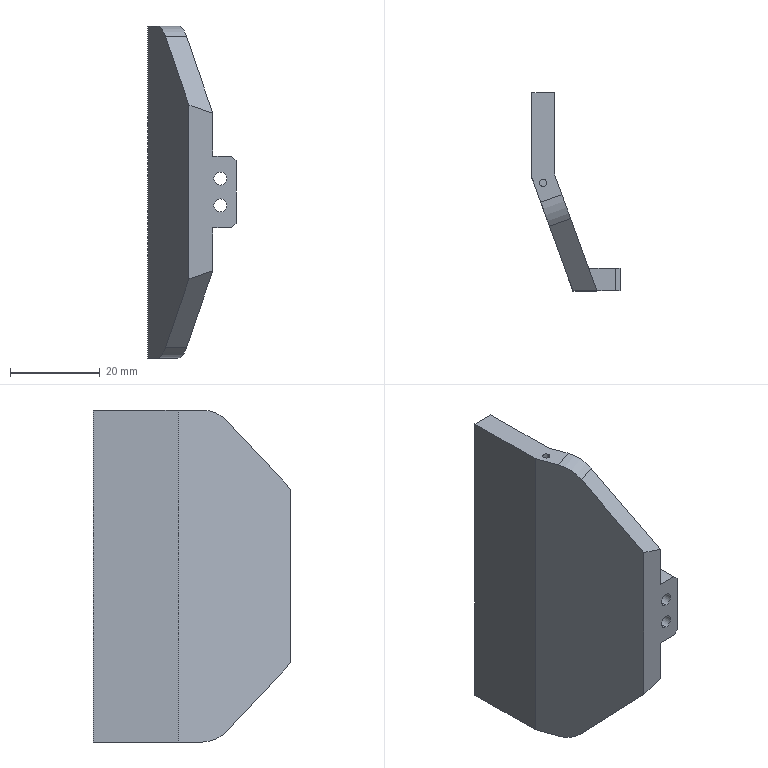NC program | NX | posted with a generic post | part box 19.643 x 44.061 x 74 mm
Lines 614 to 1768 of 4832:
(CURVE_DRIVE , TOOL : R1)
N1202 T04 M6
N1204 G54
N1206 G17 G0 G90 X15.026 Y-7.76 B0. C0. S6500 M3
N1208 G43 Z29.368 H4
N1210 Z2.364
N1212 G94 G1 Z0.531 F2500.
N1214 Y-7.722 Z0.393
N1216 Y-7.705 Z0.252
N1218 Y-7.708 Z0.109
N1220 Y-7.731 Z-0.032
N1222 Y-7.774 Z-0.168
N1224 Y-7.836 Z-0.296
N1226 Y-7.915 Z-0.415
N1228 Y-8.011 Z-0.521
N1230 Y-8.121 Z-0.612
N1232 Y-8.242 Z-0.687
N1234 Y-8.373 Z-0.743
N1236 Y-8.42 Z-0.76
N1238 X15.006 Z-0.768
N1240 X14.979 Y-8.401 Z-0.771
N1242 Y-8.348 Z-0.751
N1244 Y-8.326 Z-0.743
N1246 X14.932 Y-8.279
N1248 Y-8.302 Z-0.751
N1250 Y-8.367 Z-0.776
N1252 X14.885 Y-8.334 Z-0.782
N1254 Y-8.256 Z-0.752
N1256 Y-8.232 Z-0.743
N1258 X14.837 Y-8.185
N1260 Y-8.236 Z-0.762
N1262 Y-8.302 Z-0.787
N1264 X14.79 Y-8.27 Z-0.792
N1266 Y-8.162 Z-0.752
N1268 Y-8.137 Z-0.743
N1270 X14.743 Y-8.09
N1272 Y-8.239 Z-0.797
N1274 X14.696 Y-8.207 Z-0.803
N1276 Y-8.043 Z-0.743
N1278 X14.648 Y-7.995
N1280 Y-8.178 Z-0.81
N1282 X14.601 Y-8.149 Z-0.817
N1284 Y-7.948 Z-0.743
N1286 X14.554 Y-7.901
N1288 Y-8.12 Z-0.823
N1290 X14.507 Y-8.092 Z-0.831
N1292 Y-8.036 Z-0.809
N1294 Y-7.854 Z-0.743
N1296 X14.459 Y-7.806
N1298 Y-7.989 Z-0.81
N1300 Y-8.065 Z-0.838
N1302 X14.412 Y-8.038 Z-0.845
N1304 Y-7.943 Z-0.81
N1306 Y-7.759 Z-0.743
N1308 X14.365 Y-7.712
N1310 Y-7.931 Z-0.823
N1312 Y-8.013 Z-0.853
N1314 X14.318 Y-7.989 Z-0.862
N1316 Y-7.931 Z-0.84
N1318 Y-7.665 Z-0.743
N1320 X14.27 Y-7.617
N1322 Y-7.956 Z-0.866
N1324 Y-7.964 Z-0.87
N1326 X14.223 Y-7.94 Z-0.878
N1328 Y-7.909 Z-0.866
N1330 Y-7.57 Z-0.743
N1332 X14.176 Y-7.523
N1334 Y-7.863 Z-0.867
N1336 Y-7.917 Z-0.887
N1338 X14.129 Y-7.894 Z-0.896
N1340 Y-7.816 Z-0.867
N1342 Y-7.476 Z-0.743
N1344 X14.082 Y-7.428
N1346 Y-7.779 Z-0.87
N1348 Y-7.872 Z-0.906
N1350 X14.034 Y-7.851 Z-0.915
N1352 Y-7.779 Z-0.888
N1354 Y-7.381 Z-0.743
N1356 X13.987 Y-7.334
N1358 Y-7.779 Z-0.905
N1360 Y-7.831 Z-0.925
N1362 X13.94 Y-7.81 Z-0.934
N1364 Y-7.779 Z-0.922
N1366 Y-7.287 Z-0.743
N1368 X13.892 Y-7.239
N1370 Y-7.791 Z-0.944
N1372 X13.845 Y-7.771 Z-0.954
N1374 Y-7.192 Z-0.743
N1376 X13.798 Y-7.145
N1378 Y-7.643 Z-0.924
N1380 Y-7.752 Z-0.965
N1382 X13.779 Y-7.744 Z-0.969
N1384 X13.751 Y-7.734 Z-0.975
N1386 Y-7.097 Z-0.743
N1388 X13.703 Y-7.05
N1390 Y-7.718 Z-0.986
N1392 X13.656 Y-7.701 Z-0.997
N1394 Y-7.003 Z-0.743
N1396 X13.609 Y-6.956
N1398 Y-7.685 Z-1.008
N1400 X13.561 Y-7.669 Z-1.02
N1402 Y-6.908 Z-0.743
N1404 X13.514 Y-6.861
N1406 Y-7.654 Z-1.032
N1408 X13.467 Y-7.639 Z-1.044
N1410 Y-7.626 Z-1.039
N1412 Y-6.814 Z-0.743
N1414 X13.42 Y-6.766
N1416 Y-7.625 Z-1.056
N1418 X13.372 Y-7.61 Z-1.068
N1420 Y-6.719 Z-0.743
N1422 X13.325 Y-6.672
N1424 Y-7.486 Z-1.039
N1426 Y-7.596 Z-1.08
N1428 X13.303 Y-7.59 Z-1.086
N1430 X13.278 Y-7.584 Z-1.092
N1432 Y-6.625 Z-0.743
N1434 X13.231 Y-6.577
N1436 Y-7.572 Z-1.105
N1438 X13.183 Y-7.561 Z-1.118
N1440 Y-6.53 Z-0.743
N1442 X13.136 Y-6.483
N1444 Y-7.549 Z-1.131
N1446 X13.089 Y-7.539 Z-1.145
N1448 Y-6.435 Z-0.743
N1450 X13.041 Y-6.388
N1452 Y-7.474 Z-1.138
N1454 Y-7.528 Z-1.158
N1456 X12.994 Y-7.518 Z-1.172
N1458 Y-6.341 Z-0.743
N1460 X12.947 Y-6.294
N1462 Y-7.509 Z-1.186
N1464 X12.899 Y-7.5 Z-1.2
N1466 Y-6.246 Z-0.743
N1468 X12.852 Y-6.199
N1470 Y-7.474 Z-1.207
N1472 Y-7.492 Z-1.214
N1474 X12.805 Y-7.484 Z-1.228
N1476 Y-6.152 Z-0.743
N1478 X12.758 Y-6.104
N1480 Y-7.477 Z-1.243
N1482 X12.71 Y-7.469 Z-1.257
N1484 Y-6.102 Z-0.759
N1486 Y-6.057 Z-0.744
N1488 X12.663 Y-6.01 Z-0.743
N1490 Y-6.102 Z-0.776
N1492 Y-7.463 Z-1.272
N1494 X12.616 Y-7.457 Z-1.287
N1496 Y-5.963 Z-0.743
N1498 X12.568 Y-5.915 Z-0.744
N1500 Y-5.949 Z-0.755
N1502 Y-7.451 Z-1.302
N1504 X12.521 Y-7.445 Z-1.317
N1506 Y-5.928 Z-0.765
N1508 Y-5.867 Z-0.744
N1510 X12.474 Y-5.82
N1512 Y-5.882 Z-0.765
N1514 Y-7.406 Z-1.32
N1516 Y-7.441 Z-1.333
N1518 X12.427 Y-7.436 Z-1.349
N1520 Y-7.321 Z-1.306
N1522 Y-5.835 Z-0.766
N1524 Y-5.773 Z-0.744
N1526 X12.379 Y-5.726
N1528 Y-5.789 Z-0.766
N1530 Y-7.321 Z-1.324
N1532 Y-7.432 Z-1.365
N1534 X12.332 Y-7.429 Z-1.381
N1536 Y-7.321 Z-1.341
N1538 Y-5.742 Z-0.766
N1540 Y-5.678 Z-0.744
N1542 X12.285 Y-5.631
N1544 Y-5.696 Z-0.766
N1546 Y-7.373 Z-1.377
N1548 Y-7.426 Z-1.397
N1550 X12.238 Y-7.424 Z-1.413
N1552 Y-7.325 Z-1.377
N1554 Y-5.65 Z-0.767
N1556 Y-5.584 Z-0.744
N1558 X12.191 Y-5.537
N1560 Y-5.603 Z-0.767
N1562 Y-7.321 Z-1.392
N1564 Y-7.422 Z-1.43
N1566 X12.144 Y-7.42 Z-1.447
N1568 Y-7.321 Z-1.409
N1570 Y-5.557 Z-0.767
N1572 Y-5.49 Z-0.744
N1574 X12.096 Y-5.443
N1576 Y-5.51 Z-0.767
N1578 Y-7.34 Z-1.433
N1580 Y-7.419 Z-1.463
N1582 X12.049 Y-7.418 Z-1.48
N1584 Y-7.321 Z-1.444
N1586 Y-5.464 Z-0.768
N1588 Y-5.395 Z-0.744
N1590 X12.002 Y-5.348
N1592 Y-5.417 Z-0.768
N1594 Y-7.321 Z-1.461
N1596 Y-7.417 Z-1.497
N1598 X11.955 Z-1.514
N1600 Y-7.321 Z-1.478
N1602 Y-5.371 Z-0.768
N1604 Y-5.301 Z-0.744
N1606 X11.907 Y-5.254
N1608 Y-5.324 Z-0.768
N1610 Y-7.321 Z-1.495
N1612 Y-7.416 Z-1.531
N1614 X11.86 Z-1.548
N1616 Y-7.321 Z-1.513
N1618 Y-5.278 Z-0.769
N1620 Y-5.206 Z-0.744
N1622 X11.813 Y-5.159
N1624 Y-5.231 Z-0.769
N1626 Y-7.321 Z-1.53
N1628 Y-7.416 Z-1.566
N1630 X11.766 Z-1.583
N1632 Y-7.321 Z-1.547
N1634 Y-5.184 Z-0.769
N1636 Y-5.112 Z-0.744
N1638 X11.718 Y-5.064
N1640 Y-5.138 Z-0.769
N1642 Y-7.321 Z-1.564
N1644 Y-7.416 Z-1.6
N1646 X11.671 Z-1.617
N1648 Y-7.321 Z-1.581
N1650 Y-5.091 Z-0.77
N1652 Y-5.017 Z-0.744
N1654 X11.624 Y-4.97
N1656 Y-5.045 Z-0.77
N1658 Y-7.321 Z-1.599
N1660 Y-7.416 Z-1.634
N1662 X11.576 Z-1.652
N1664 Y-7.321 Z-1.616
N1666 Y-4.998 Z-0.77
N1668 Y-4.922 Z-0.744
N1670 X11.529 Y-4.875
N1672 Y-4.952 Z-0.771
N1674 Y-7.321 Z-1.633
N1676 Y-7.416 Z-1.669
N1678 X11.482 Z-1.686
N1680 Y-7.321 Z-1.65
N1682 Y-4.905 Z-0.771
N1684 Y-4.828 Z-0.744
N1686 X11.435 Y-4.781
N1688 Y-4.859 Z-0.771
N1690 Y-7.321 Z-1.667
N1692 Y-7.416 Z-1.703
N1694 X11.387 Y-7.417 Z-1.72
N1696 Y-7.321 Z-1.684
N1698 Y-4.812 Z-0.771
N1700 Y-4.734 Z-0.744
N1702 X11.353 Y-4.699 Z-0.743
N1704 X11.341 Y-4.685
N1706 Y-4.766 Z-0.771
N1708 Y-6.434 Z-1.378
N1710 Y-7.321 Z-1.701
N1712 Y-7.417 Z-1.737
N1714 X11.293 Y-7.418 Z-1.753
N1716 Y-7.321 Z-1.717
N1718 Y-5.106 Z-0.911
N1720 Y-4.719 Z-0.771
N1722 Y-4.63 Z-0.739
N1724 X11.246 Y-4.577 Z-0.735
N1726 Y-4.825 Z-0.825
N1728 Y-7.321 Z-1.733
N1730 Y-7.419 Z-1.769
N1732 X11.198 Y-7.42 Z-1.785
N1734 Y-7.321 Z-1.748
N1736 Y-4.626 Z-0.768
N1738 Y-4.526 Z-0.732
N1740 X11.151 Y-4.476 Z-0.729
N1742 Y-4.579 Z-0.766
N1744 Y-7.323 Z-1.765
N1746 Y-7.42 Z-1.801
N1748 X11.103 Y-7.422 Z-1.815
N1750 Y-7.321 Z-1.777
N1752 Y-6.559 Z-1.5
N1754 Y-6.407 Z-1.445
N1756 Y-6.361 Z-1.428
N1758 Y-4.532 Z-0.762
N1760 Y-4.429 Z-0.725
N1762 X11.078 Y-4.404
N1764 X11.063 Y-4.391
N1766 X11.055 Y-4.383 Z-0.724
N1768 Y-4.395 Z-0.728
N1770 Y-4.425 Z-0.737
N1772 Y-6.314 Z-1.424
N1774 Y-6.374 Z-1.447
N1776 Y-6.559 Z-1.513
N1778 Y-7.321 Z-1.791
N1780 Y-7.423 Z-1.829
N1782 X11.006 Y-7.424 Z-1.842
N1784 Y-7.321 Z-1.804
N1786 Y-4.425 Z-0.75
N1788 Y-4.34 Z-0.721
N1790 X10.982 Y-4.319 Z-0.719
N1792 X10.958 Y-4.3 Z-0.717
N1794 Y-4.389 Z-0.749
N1796 Y-7.321 Z-1.816
N1798 Y-7.425 Z-1.855
N1800 X10.909 Y-7.426 Z-1.866
N1802 Y-7.321 Z-1.827
N1804 Y-4.342 Z-0.743
N1806 Y-4.261 Z-0.715
N1808 X10.861 Y-4.223 Z-0.712
N1810 Y-7.321 Z-1.839
N1812 Y-7.427 Z-1.878
N1814 X10.828 Z-1.886
N1816 X10.812 Y-7.428 Z-1.889
N1818 Y-7.321 Z-1.849
N1820 Y-4.189 Z-0.71
N1822 X10.763 Y-4.158 Z-0.708
N1824 Y-7.321 Z-1.859
N1826 Y-7.428 Z-1.898
N1828 X10.714 Y-7.429 Z-1.908
N1830 Y-7.321 Z-1.868
N1832 Y-4.127 Z-0.706
N1834 X10.671 Y-4.1 Z-0.704
N1836 X10.665 Y-4.097
N1838 Y-4.12 Z-0.711
N1840 Y-7.321 Z-1.877
N1842 Y-7.43 Z-1.917
N1844 X10.615 Z-1.925
N1846 Y-7.321 Z-1.884
N1848 Y-4.12 Z-0.719
N1850 Y-4.072 Z-0.703
N1852 X10.595 Y-4.062 Z-0.702
N1854 X10.566 Y-4.049 Z-0.701
N1856 Y-4.12 Z-0.726
N1858 Y-7.321 Z-1.891
N1860 Y-7.431 Z-1.932
N1862 X10.518 Y-7.432 Z-1.939
N1864 X10.516
N1866 Y-7.321 Z-1.898
N1868 Y-4.12 Z-0.733
N1870 Y-4.028 Z-0.7
N1872 X10.467 Y-4.011
N1874 Y-4.12 Z-0.738
N1876 Y-7.321 Z-1.903
N1878 Y-7.432 Z-1.944
N1880 X10.417 Z-1.949
N1882 Y-7.321 Z-1.908
N1884 Y-4.12 Z-0.743
N1886 Y-3.994 Z-0.698
N1888 X10.367 Y-3.977 Z-0.696
N1890 Y-7.321 Z-1.913
N1892 Y-7.433 Z-1.954
N1894 X10.317 Z-1.958
N1896 Y-7.321 Z-1.916
N1898 Y-3.965 Z-0.695
N1900 X10.267 Y-3.952 Z-0.694
N1902 Y-7.321 Z-1.919
N1904 Y-7.433 Z-1.961
N1906 X10.218 Y-7.434 Z-1.964
N1908 Y-7.321 Z-1.922
N1910 Y-3.967 Z-0.702
N1912 Y-3.944 Z-0.694
N1914 X10.209 Y-3.943
N1916 X10.168 Y-3.941
N1918 Y-7.321 Z-1.924
N1920 Y-7.434 Z-1.965
N1922 X10.118 Z-1.967
N1924 Y-7.321 Z-1.925
N1926 Y-3.938 Z-0.694
N1928 X10.068 Y-3.936 Z-0.695
N1930 Y-3.967 Z-0.706
N1932 Y-7.324 Z-1.927
N1934 Y-7.434 Z-1.968
N1936 X10.018
N1938 Y-7.321 Z-1.927
N1940 Y-3.967 Z-0.706
N1942 Y-3.935 Z-0.695
N1944 X9.968
N1946 Y-3.967 Z-0.706
N1948 Y-7.321 Z-1.927
N1950 Y-7.434 Z-1.968
N1952 X9.918
N1954 Y-7.321 Z-1.927
N1956 Y-3.967 Z-0.706
N1958 Y-3.935 Z-0.695
N1960 X9.868
N1962 Y-3.967 Z-0.706
N1964 Y-7.321 Z-1.927
N1966 Y-7.434 Z-1.968
N1968 X9.818
N1970 Y-7.321 Z-1.927
N1972 Y-3.967 Z-0.706
N1974 Y-3.935 Z-0.695
N1976 X9.768
N1978 Y-3.967 Z-0.706
N1980 Y-7.321 Z-1.927
N1982 Y-7.434 Z-1.968
N1984 X9.718
N1986 Y-7.321 Z-1.927
N1988 Y-3.967 Z-0.706
N1990 Y-3.935 Z-0.695
N1992 X9.668
N1994 Y-3.967 Z-0.706
N1996 Y-7.321 Z-1.927
N1998 Y-7.434 Z-1.968
N2000 X9.618
N2002 Y-7.321 Z-1.927
N2004 Y-3.967 Z-0.706
N2006 Y-3.935 Z-0.695
N2008 X9.568
N2010 Y-3.967 Z-0.706
N2012 Y-7.321 Z-1.927
N2014 Y-7.434 Z-1.968
N2016 X9.518
N2018 Y-7.321 Z-1.927
N2020 Y-3.967 Z-0.706
N2022 Y-3.935 Z-0.695
N2024 X9.468
N2026 Y-3.967 Z-0.706
N2028 Y-7.321 Z-1.927
N2030 Y-7.434 Z-1.968
N2032 X9.418
N2034 Y-7.321 Z-1.927
N2036 Y-3.967 Z-0.706
N2038 Y-3.935 Z-0.695
N2040 X9.368
N2042 Y-3.967 Z-0.706
N2044 Y-7.321 Z-1.927
N2046 Y-7.434 Z-1.968
N2048 X9.318
N2050 Y-7.321 Z-1.927
N2052 Y-3.967 Z-0.706
N2054 Y-3.935 Z-0.695
N2056 X9.268
N2058 Y-3.967 Z-0.706
N2060 Y-7.321 Z-1.927
N2062 Y-7.434 Z-1.968
N2064 X9.218
N2066 Y-7.321 Z-1.927
N2068 Y-3.967 Z-0.706
N2070 Y-3.935 Z-0.695
N2072 X9.168
N2074 Y-3.967 Z-0.706
N2076 Y-7.321 Z-1.927
N2078 Y-7.434 Z-1.968
N2080 X9.118
N2082 Y-7.321 Z-1.927
N2084 Y-3.967 Z-0.706
N2086 Y-3.935 Z-0.695
N2088 X9.068
N2090 Y-3.967 Z-0.706
N2092 Y-7.321 Z-1.927
N2094 Y-7.434 Z-1.968
N2096 X9.018
N2098 Y-7.321 Z-1.927
N2100 Y-3.967 Z-0.706
N2102 Y-3.935 Z-0.695
N2104 X8.968
N2106 Y-3.967 Z-0.706
N2108 Y-7.321 Z-1.927
N2110 Y-7.434 Z-1.968
N2112 X8.918
N2114 Y-7.321 Z-1.927
N2116 Y-3.967 Z-0.706
N2118 Y-3.935 Z-0.695
N2120 X8.868
N2122 Y-3.967 Z-0.706
N2124 Y-7.321 Z-1.927
N2126 Y-7.434 Z-1.968
N2128 X8.818
N2130 Y-7.321 Z-1.927
N2132 Y-3.967 Z-0.706
N2134 Y-3.935 Z-0.695
N2136 X8.768
N2138 Y-3.967 Z-0.706
N2140 Y-7.321 Z-1.927
N2142 Y-7.434 Z-1.968
N2144 X8.718
N2146 Y-7.321 Z-1.927
N2148 Y-3.967 Z-0.706
N2150 Y-3.935 Z-0.695
N2152 X8.668
N2154 Y-3.967 Z-0.706
N2156 Y-7.321 Z-1.927
N2158 Y-7.434 Z-1.968
N2160 X8.618
N2162 Y-7.321 Z-1.927
N2164 Y-3.967 Z-0.706
N2166 Y-3.935 Z-0.695
N2168 X8.568
N2170 Y-3.967 Z-0.706
N2172 Y-7.321 Z-1.927
N2174 Y-7.434 Z-1.968
N2176 X8.518
N2178 Y-7.323 Z-1.927
N2180 Y-3.969 Z-0.706
N2182 Y-3.935 Z-0.695
N2184 X8.468
N2186 Y-3.967 Z-0.706
N2188 Y-7.321 Z-1.927
N2190 Y-7.434 Z-1.968
N2192 X8.418
N2194 Y-7.321 Z-1.927
N2196 Y-3.967 Z-0.706
N2198 Y-3.935 Z-0.695
N2200 X8.368
N2202 Y-3.967 Z-0.706
N2204 Y-7.326 Z-1.928
N2206 Y-7.434 Z-1.968
N2208 X8.318
N2210 Y-7.321 Z-1.927
N2212 Y-3.967 Z-0.706
N2214 Y-3.935 Z-0.695
N2216 X8.268
N2218 Y-3.967 Z-0.706
N2220 Y-7.321 Z-1.927
N2222 Y-7.434 Z-1.968
N2224 X8.218
N2226 Y-7.321 Z-1.927
N2228 Y-3.967 Z-0.706
N2230 Y-3.935 Z-0.695
N2232 X8.168
N2234 Y-3.967 Z-0.706
N2236 Y-7.321 Z-1.927
N2238 Y-7.434 Z-1.968
N2240 X8.118
N2242 Y-7.321 Z-1.927
N2244 Y-3.967 Z-0.706
N2246 Y-3.935 Z-0.695
N2248 X8.068
N2250 Y-3.967 Z-0.706
N2252 Y-7.321 Z-1.927
N2254 Y-7.434 Z-1.968
N2256 X8.018
N2258 Y-7.321 Z-1.927
N2260 Y-3.967 Z-0.706
N2262 Y-3.935 Z-0.695
N2264 X7.968
N2266 Y-3.967 Z-0.706
N2268 Y-7.321 Z-1.927
N2270 Y-7.434 Z-1.968
N2272 X7.918
N2274 Y-7.321 Z-1.927
N2276 Y-3.967 Z-0.706
N2278 Y-3.935 Z-0.695
N2280 X7.868
N2282 Y-3.967 Z-0.706
N2284 Y-7.321 Z-1.927
N2286 Y-7.434 Z-1.968
N2288 X7.818
N2290 Y-7.321 Z-1.927
N2292 Y-3.967 Z-0.706
N2294 Y-3.935 Z-0.695
N2296 X7.768
N2298 Y-3.967 Z-0.706
N2300 Y-7.321 Z-1.927
N2302 Y-7.434 Z-1.968
N2304 X7.718
N2306 Y-7.321 Z-1.927
N2308 Y-3.967 Z-0.706
N2310 Y-3.935 Z-0.695
N2312 X7.668
N2314 Y-3.967 Z-0.706
N2316 Y-7.321 Z-1.927
N2318 Y-7.434 Z-1.968
N2320 X7.618
N2322 Y-7.321 Z-1.927
N2324 Y-3.967 Z-0.706
N2326 Y-3.935 Z-0.695
N2328 X7.568
N2330 Y-3.967 Z-0.706
N2332 Y-7.321 Z-1.927
N2334 Y-7.434 Z-1.968
N2336 X7.518
N2338 Y-7.321 Z-1.927
N2340 Y-3.967 Z-0.706
N2342 Y-3.935 Z-0.695
N2344 X7.468
N2346 Y-3.967 Z-0.706
N2348 Y-7.321 Z-1.927
N2350 Y-7.434 Z-1.968
N2352 X7.418
N2354 Y-7.321 Z-1.927
N2356 Y-3.967 Z-0.706
N2358 Y-3.935 Z-0.695
N2360 X7.368
N2362 Y-3.967 Z-0.706
N2364 Y-7.321 Z-1.927
N2366 Y-7.434 Z-1.968
N2368 X7.318
N2370 Y-7.321 Z-1.927
N2372 Y-3.967 Z-0.706
N2374 Y-3.935 Z-0.695
N2376 X7.268
N2378 Y-3.967 Z-0.706
N2380 Y-7.321 Z-1.927
N2382 Y-7.434 Z-1.968
N2384 X7.218
N2386 Y-7.321 Z-1.927
N2388 Y-3.967 Z-0.706
N2390 Y-3.935 Z-0.695
N2392 X7.168
N2394 Y-3.967 Z-0.706
N2396 Y-7.321 Z-1.927
N2398 Y-7.434 Z-1.968
N2400 X7.118
N2402 Y-7.321 Z-1.927
N2404 Y-3.967 Z-0.706
N2406 Y-3.935 Z-0.695
N2408 X7.068
N2410 Y-3.967 Z-0.706
N2412 Y-7.321 Z-1.927
N2414 Y-7.434 Z-1.968
N2416 X7.018
N2418 Y-7.321 Z-1.927
N2420 Y-3.967 Z-0.706
N2422 Y-3.935 Z-0.695
N2424 X6.968
N2426 Y-3.967 Z-0.706
N2428 Y-7.326 Z-1.928
N2430 Y-7.434 Z-1.968
N2432 X6.918
N2434 Y-7.321 Z-1.927
N2436 Y-3.967 Z-0.706
N2438 Y-3.935 Z-0.695
N2440 X6.868
N2442 Y-3.967 Z-0.706
N2444 Y-7.321 Z-1.927
N2446 Y-7.434 Z-1.968
N2448 X6.818
N2450 Y-7.326 Z-1.928
N2452 Y-3.967 Z-0.706
N2454 Y-3.935 Z-0.695
N2456 X6.768
N2458 Y-3.967 Z-0.706
N2460 Y-7.321 Z-1.927
N2462 Y-7.434 Z-1.968
N2464 X6.718
N2466 Y-7.321 Z-1.927
N2468 Y-3.967 Z-0.706
N2470 Y-3.935 Z-0.695
N2472 X6.668
N2474 Y-3.967 Z-0.706
N2476 Y-7.321 Z-1.927
N2478 Y-7.434 Z-1.968
N2480 X6.618
N2482 Y-7.321 Z-1.927
N2484 Y-3.967 Z-0.706
N2486 Y-3.935 Z-0.695
N2488 X6.568
N2490 Y-3.967 Z-0.706
N2492 Y-7.321 Z-1.927
N2494 Y-7.434 Z-1.968
N2496 X6.518
N2498 Y-7.321 Z-1.927
N2500 Y-3.967 Z-0.706
N2502 Y-3.935 Z-0.695
N2504 X6.468
N2506 Y-3.967 Z-0.706
N2508 Y-7.321 Z-1.927
N2510 Y-7.434 Z-1.968
N2512 X6.418
N2514 Y-7.321 Z-1.927
N2516 Y-3.967 Z-0.706
N2518 Y-3.935 Z-0.695
N2520 X6.368
N2522 Y-3.967 Z-0.706
N2524 Y-7.321 Z-1.927
N2526 Y-7.434 Z-1.968
N2528 X6.318
N2530 Y-7.321 Z-1.927
N2532 Y-3.967 Z-0.706
N2534 Y-3.935 Z-0.695
N2536 X6.268
N2538 Y-3.967 Z-0.706
N2540 Y-7.321 Z-1.927
N2542 Y-7.434 Z-1.968
N2544 X6.218
N2546 Y-7.321 Z-1.927
N2548 Y-3.967 Z-0.706
N2550 Y-3.935 Z-0.695
N2552 X6.168
N2554 Y-3.967 Z-0.706
N2556 Y-7.321 Z-1.927
N2558 Y-7.434 Z-1.968
N2560 X6.118
N2562 Y-7.321 Z-1.927
N2564 Y-3.967 Z-0.706
N2566 Y-3.935 Z-0.695
N2568 X6.068
N2570 Y-3.967 Z-0.706
N2572 Y-7.321 Z-1.927
N2574 Y-7.434 Z-1.968
N2576 X6.018
N2578 Y-7.321 Z-1.927
N2580 Y-3.967 Z-0.706
N2582 Y-3.935 Z-0.695
N2584 X5.968
N2586 Y-3.967 Z-0.706
N2588 Y-7.321 Z-1.927
N2590 Y-7.434 Z-1.968
N2592 X5.918
N2594 Y-7.321 Z-1.927
N2596 Y-3.967 Z-0.706
N2598 Y-3.935 Z-0.695
N2600 X5.868
N2602 Y-3.967 Z-0.706
N2604 Y-7.321 Z-1.927
N2606 Y-7.434 Z-1.968
N2608 X5.818
N2610 Y-7.321 Z-1.927
N2612 Y-3.967 Z-0.706
N2614 Y-3.935 Z-0.695
N2616 X5.768
N2618 Y-3.967 Z-0.706
N2620 Y-7.321 Z-1.927
N2622 Y-7.434 Z-1.968
N2624 X5.718
N2626 Y-7.321 Z-1.927
N2628 Y-3.967 Z-0.706
N2630 Y-3.935 Z-0.695
N2632 X5.668
N2634 Y-3.967 Z-0.706
N2636 Y-7.321 Z-1.927
N2638 Y-7.434 Z-1.968
N2640 X5.618
N2642 Y-7.321 Z-1.927
N2644 Y-3.967 Z-0.706
N2646 Y-3.935 Z-0.695
N2648 X5.568
N2650 Y-3.967 Z-0.706
N2652 Y-7.321 Z-1.927
N2654 Y-7.434 Z-1.968
N2656 X5.518
N2658 Y-7.321 Z-1.927
N2660 Y-3.967 Z-0.706
N2662 Y-3.935 Z-0.695
N2664 X5.468
N2666 Y-3.967 Z-0.706
N2668 Y-7.321 Z-1.927
N2670 Y-7.434 Z-1.968
N2672 X5.418
N2674 Y-7.321 Z-1.927
N2676 Y-3.967 Z-0.706
N2678 Y-3.935 Z-0.695
N2680 X5.368
N2682 Y-3.967 Z-0.706
N2684 Y-7.321 Z-1.927
N2686 Y-7.434 Z-1.968
N2688 X5.318
N2690 Y-7.321 Z-1.927
N2692 Y-3.967 Z-0.706
N2694 Y-3.935 Z-0.695
N2696 X5.268
N2698 Y-3.967 Z-0.706
N2700 Y-7.324 Z-1.928
N2702 Y-7.434 Z-1.968
N2704 X5.218
N2706 Y-7.321 Z-1.927
N2708 Y-3.967 Z-0.706
N2710 Y-3.935 Z-0.695
N2712 X5.168
N2714 Y-3.967 Z-0.706
N2716 Y-7.321 Z-1.927
N2718 Y-7.434 Z-1.968
N2720 X5.118
N2722 Y-7.321 Z-1.927
N2724 Y-3.967 Z-0.706
N2726 Y-3.935 Z-0.695
N2728 X5.068
N2730 Y-3.967 Z-0.706
N2732 Y-7.321 Z-1.927
N2734 Y-7.434 Z-1.968
N2736 X5.018
N2738 Y-7.321 Z-1.927
N2740 Y-3.967 Z-0.706
N2742 Y-3.935 Z-0.695
N2744 X4.968
N2746 Y-3.967 Z-0.706
N2748 Y-7.321 Z-1.927
N2750 Y-7.434 Z-1.968
N2752 X4.918
N2754 Y-7.321 Z-1.927
N2756 Y-3.967 Z-0.706
N2758 Y-3.935 Z-0.695
N2760 X4.868
N2762 Y-3.967 Z-0.706
N2764 Y-7.321 Z-1.927
N2766 Y-7.434 Z-1.968
N2768 X4.818
N2770 Y-7.321 Z-1.927
N2772 Y-3.967 Z-0.706
N2774 Y-3.935 Z-0.695
N2776 X4.768
N2778 Y-3.967 Z-0.706
N2780 Y-7.321 Z-1.927
N2782 Y-7.434 Z-1.968
N2784 X4.718
N2786 Y-7.321 Z-1.927
N2788 Y-3.967 Z-0.706
N2790 Y-3.935 Z-0.695
N2792 X4.668
N2794 Y-3.967 Z-0.706
N2796 Y-7.321 Z-1.927
N2798 Y-7.434 Z-1.968
N2800 X4.618
N2802 Y-7.321 Z-1.927
N2804 Y-3.967 Z-0.706
N2806 Y-3.935 Z-0.695
N2808 X4.568
N2810 Y-3.967 Z-0.706
N2812 Y-7.321 Z-1.927
N2814 Y-7.434 Z-1.968
N2816 X4.518
N2818 Y-7.321 Z-1.927
N2820 Y-3.967 Z-0.706
N2822 Y-3.935 Z-0.695
N2824 X4.468
N2826 Y-3.967 Z-0.706
N2828 Y-7.321 Z-1.927
N2830 Y-7.434 Z-1.968
N2832 X4.418
N2834 Y-7.321 Z-1.927
N2836 Y-3.967 Z-0.706
N2838 Y-3.935 Z-0.695
N2840 X4.368
N2842 Y-3.967 Z-0.706
N2844 Y-7.321 Z-1.927
N2846 Y-7.434 Z-1.968
N2848 X4.318
N2850 Y-7.321 Z-1.927
N2852 Y-3.967 Z-0.706
N2854 Y-3.935 Z-0.695
N2856 X4.268
N2858 Y-3.967 Z-0.706
N2860 Y-7.321 Z-1.927
N2862 Y-7.434 Z-1.968
N2864 X4.218
N2866 Y-7.321 Z-1.927
N2868 Y-3.967 Z-0.706
N2870 Y-3.935 Z-0.695
N2872 X4.168
N2874 Y-3.967 Z-0.706
N2876 Y-7.321 Z-1.927
N2878 Y-7.434 Z-1.968
N2880 X4.118
N2882 Y-7.321 Z-1.927
N2884 Y-3.967 Z-0.706
N2886 Y-3.935 Z-0.695
N2888 X4.068
N2890 Y-3.967 Z-0.706
N2892 Y-7.321 Z-1.927
N2894 Y-7.434 Z-1.968
N2896 X4.018
N2898 Y-7.321 Z-1.927
N2900 Y-3.967 Z-0.706
N2902 Y-3.935 Z-0.695
N2904 X3.968
N2906 Y-3.967 Z-0.706
N2908 Y-7.321 Z-1.927
N2910 Y-7.434 Z-1.968
N2912 X3.918
N2914 Y-7.321 Z-1.927
N2916 Y-3.967 Z-0.706
N2918 Y-3.935 Z-0.695
N2920 X3.868
N2922 Y-3.967 Z-0.706
N2924 Y-7.321 Z-1.927
N2926 Y-7.434 Z-1.968
N2928 X3.818
N2930 Y-7.321 Z-1.927
N2932 Y-3.967 Z-0.706
N2934 Y-3.935 Z-0.695
N2936 X3.768
N2938 Y-3.967 Z-0.706
N2940 Y-7.321 Z-1.927
N2942 Y-7.434 Z-1.968
N2944 X3.718
N2946 Y-7.323 Z-1.927
N2948 Y-3.969 Z-0.706
N2950 Y-3.935 Z-0.695
N2952 X3.668
N2954 Y-3.967 Z-0.706
N2956 Y-7.321 Z-1.927
N2958 Y-7.434 Z-1.968
N2960 X3.618
N2962 Y-7.321 Z-1.927
N2964 Y-3.967 Z-0.706
N2966 Y-3.935 Z-0.695
N2968 X3.568
N2970 Y-3.967 Z-0.706
N2972 Y-7.326 Z-1.928
N2974 Y-7.434 Z-1.968
N2976 X3.518
N2978 Y-7.321 Z-1.927
N2980 Y-3.967 Z-0.706
N2982 Y-3.935 Z-0.695
N2984 X3.468
N2986 Y-3.967 Z-0.706
N2988 Y-7.321 Z-1.927
N2990 Y-7.434 Z-1.968
N2992 X3.418
N2994 Y-7.321 Z-1.927
N2996 Y-3.967 Z-0.706
N2998 Y-3.935 Z-0.695
N3000 X3.368
N3002 Y-3.967 Z-0.706
N3004 Y-7.321 Z-1.927
N3006 Y-7.434 Z-1.968
N3008 X3.318
N3010 Y-7.321 Z-1.927
N3012 Y-3.967 Z-0.706
N3014 Y-3.935 Z-0.695
N3016 X3.268
N3018 Y-3.967 Z-0.706
N3020 Y-7.321 Z-1.927
N3022 Y-7.434 Z-1.968
N3024 X3.218
N3026 Y-7.321 Z-1.927
N3028 Y-3.967 Z-0.706
N3030 Y-3.935 Z-0.695
N3032 X3.168
N3034 Y-3.967 Z-0.706
N3036 Y-7.321 Z-1.927
N3038 Y-7.434 Z-1.968
N3040 X3.118
N3042 Y-7.321 Z-1.927
N3044 Y-3.967 Z-0.706
N3046 Y-3.935 Z-0.695
N3048 X3.068
N3050 Y-3.967 Z-0.706
N3052 Y-7.321 Z-1.927
N3054 Y-7.434 Z-1.968
N3056 X3.018
N3058 Y-7.321 Z-1.927
N3060 Y-3.967 Z-0.706
N3062 Y-3.935 Z-0.695
N3064 X2.968
N3066 Y-3.967 Z-0.706
N3068 Y-7.321 Z-1.927
N3070 Y-7.434 Z-1.968
N3072 X2.918
N3074 Y-7.321 Z-1.927
N3076 Y-3.967 Z-0.706
N3078 Y-3.935 Z-0.695
N3080 X2.868
N3082 Y-3.967 Z-0.706
N3084 Y-7.321 Z-1.927
N3086 Y-7.434 Z-1.968
N3088 X2.818
N3090 Y-7.321 Z-1.927
N3092 Y-3.967 Z-0.706
N3094 Y-3.935 Z-0.695
N3096 X2.768
N3098 Y-3.967 Z-0.706
N3100 Y-7.321 Z-1.927
N3102 Y-7.434 Z-1.968
N3104 X2.718
N3106 Y-7.321 Z-1.927
N3108 Y-3.967 Z-0.706
N3110 Y-3.935 Z-0.695
N3112 X2.668
N3114 Y-3.967 Z-0.706
N3116 Y-7.321 Z-1.927
N3118 Y-7.434 Z-1.968
N3120 X2.618
N3122 Y-7.321 Z-1.927
N3124 Y-3.967 Z-0.706
N3126 Y-3.935 Z-0.695
N3128 X2.568
N3130 Y-3.967 Z-0.706
N3132 Y-7.321 Z-1.927
N3134 Y-7.434 Z-1.968
N3136 X2.518
N3138 Y-7.321 Z-1.927
N3140 Y-3.967 Z-0.706
N3142 Y-3.935 Z-0.695
N3144 X2.468
N3146 Y-3.967 Z-0.706
N3148 Y-7.321 Z-1.927
N3150 Y-7.434 Z-1.968
N3152 X2.418
N3154 Y-7.321 Z-1.927
N3156 Y-3.967 Z-0.706
N3158 Y-3.935 Z-0.695
N3160 X2.368
N3162 Y-3.967 Z-0.706
N3164 Y-7.321 Z-1.927
N3166 Y-7.434 Z-1.968
N3168 X2.318
N3170 Y-7.321 Z-1.927
N3172 Y-3.967 Z-0.706
N3174 Y-3.935 Z-0.695
N3176 X2.268
N3178 Y-3.967 Z-0.706
N3180 Y-7.321 Z-1.927
N3182 Y-7.434 Z-1.968
N3184 X2.218
N3186 Y-7.321 Z-1.927
N3188 Y-3.967 Z-0.706
N3190 Y-3.935 Z-0.695
N3192 X2.168
N3194 Y-3.967 Z-0.706
N3196 Y-7.321 Z-1.927
N3198 Y-7.434 Z-1.968
N3200 X2.118
N3202 Y-7.321 Z-1.927
N3204 Y-3.967 Z-0.706
N3206 Y-3.935 Z-0.695
N3208 X2.068
N3210 Y-3.967 Z-0.706
N3212 Y-7.321 Z-1.927
N3214 Y-7.434 Z-1.968
N3216 X2.018
N3218 Y-7.326 Z-1.928
N3220 Y-3.967 Z-0.706
N3222 Y-3.935 Z-0.695
N3224 X1.968
N3226 Y-3.967 Z-0.706
N3228 Y-7.321 Z-1.927
N3230 Y-7.434 Z-1.968
N3232 X1.918
N3234 Y-7.321 Z-1.927
N3236 Y-3.967 Z-0.706
N3238 Y-3.935 Z-0.695
N3240 X1.868
N3242 Y-3.967 Z-0.706
N3244 Y-7.321 Z-1.927
N3246 Y-7.434 Z-1.968
N3248 X1.818
N3250 Y-7.321 Z-1.927
N3252 Y-3.967 Z-0.706
N3254 Y-3.935 Z-0.695
N3256 X1.768
N3258 Y-3.967 Z-0.706
N3260 Y-7.321 Z-1.927
N3262 Y-7.434 Z-1.968
N3264 X1.718
N3266 Y-7.321 Z-1.927
N3268 Y-3.967 Z-0.706
N3270 Y-3.935 Z-0.695
N3272 X1.668
N3274 Y-3.967 Z-0.706
N3276 Y-7.321 Z-1.927
N3278 Y-7.434 Z-1.968
N3280 X1.618
N3282 Y-7.321 Z-1.927
N3284 Y-3.967 Z-0.706
N3286 Y-3.935 Z-0.695
N3288 X1.568
N3290 Y-3.967 Z-0.706
N3292 Y-7.321 Z-1.927
N3294 Y-7.434 Z-1.968
N3296 X1.518
N3298 Y-7.321 Z-1.927
N3300 Y-3.967 Z-0.706
N3302 Y-3.935 Z-0.695
N3304 X1.468
N3306 Y-3.967 Z-0.706
N3308 Y-7.321 Z-1.927
N3310 Y-7.434 Z-1.968
N3312 X1.418
N3314 Y-7.321 Z-1.927
N3316 Y-3.967 Z-0.706
N3318 Y-3.935 Z-0.695
N3320 X1.368
N3322 Y-3.967 Z-0.706
N3324 Y-7.321 Z-1.927
N3326 Y-7.434 Z-1.968
N3328 X1.318
N3330 Y-7.321 Z-1.927
N3332 Y-3.967 Z-0.706
N3334 Y-3.935 Z-0.695
N3336 X1.268
N3338 Y-3.967 Z-0.706
N3340 Y-7.321 Z-1.927
N3342 Y-7.434 Z-1.968
N3344 X1.218
N3346 Y-7.321 Z-1.927
N3348 Y-3.967 Z-0.706
N3350 Y-3.935 Z-0.695
N3352 X1.168
N3354 Y-3.967 Z-0.706
N3356 Y-7.321 Z-1.927
N3358 Y-7.434 Z-1.968
N3360 X1.118
N3362 Y-7.321 Z-1.927
N3364 Y-3.967 Z-0.706
N3366 Y-3.935 Z-0.695
N3368 X1.068
N3370 Y-3.967 Z-0.706
N3372 Y-7.321 Z-1.927
N3374 Y-7.434 Z-1.968
N3376 X1.018
N3378 Y-7.321 Z-1.927
N3380 Y-3.967 Z-0.706
N3382 Y-3.935 Z-0.695
N3384 X0.968
N3386 Y-3.967 Z-0.706
N3388 Y-7.321 Z-1.927
N3390 Y-7.434 Z-1.968
N3392 X0.918
N3394 Y-7.321 Z-1.927
N3396 Y-3.967 Z-0.706
N3398 Y-3.935 Z-0.695
N3400 X0.868
N3402 Y-3.967 Z-0.706
N3404 Y-7.321 Z-1.927
N3406 Y-7.434 Z-1.968
N3408 X0.818
N3410 Y-7.321 Z-1.927
N3412 Y-3.967 Z-0.706
N3414 Y-3.935 Z-0.695
N3416 X0.768
N3418 Y-3.967 Z-0.706
N3420 Y-7.321 Z-1.927
N3422 Y-7.434 Z-1.968
N3424 X0.718
N3426 Y-7.321 Z-1.927
N3428 Y-3.967 Z-0.706
N3430 Y-3.935 Z-0.695
N3432 X0.668
N3434 Y-3.967 Z-0.706
N3436 Y-7.321 Z-1.927
N3438 Y-7.434 Z-1.968
N3440 X0.618
N3442 Y-7.321 Z-1.927
N3444 Y-3.967 Z-0.706
N3446 Y-3.935 Z-0.695
N3448 X0.568
N3450 Y-3.967 Z-0.706
N3452 Y-7.321 Z-1.927
N3454 Y-7.434 Z-1.968
N3456 X0.518
N3458 Y-7.321 Z-1.927
N3460 Y-3.967 Z-0.706
N3462 Y-3.935 Z-0.695
N3464 X0.468
N3466 Y-3.967 Z-0.706
N3468 Y-7.324 Z-1.928
N3470 Y-7.434 Z-1.968
N3472 X0.418
N3474 Y-7.321 Z-1.927
N3476 Y-3.967 Z-0.706
N3478 Y-3.935 Z-0.695
N3480 X0.368
N3482 Y-3.967 Z-0.706
N3484 Y-7.321 Z-1.927
N3486 Y-7.434 Z-1.968
N3488 X0.318
N3490 Y-7.321 Z-1.927
N3492 Y-3.967 Z-0.706
N3494 Y-3.935 Z-0.695
N3496 X0.268
N3498 Y-3.967 Z-0.706
N3500 Y-7.321 Z-1.927
N3502 Y-7.434 Z-1.968
N3504 X0.218